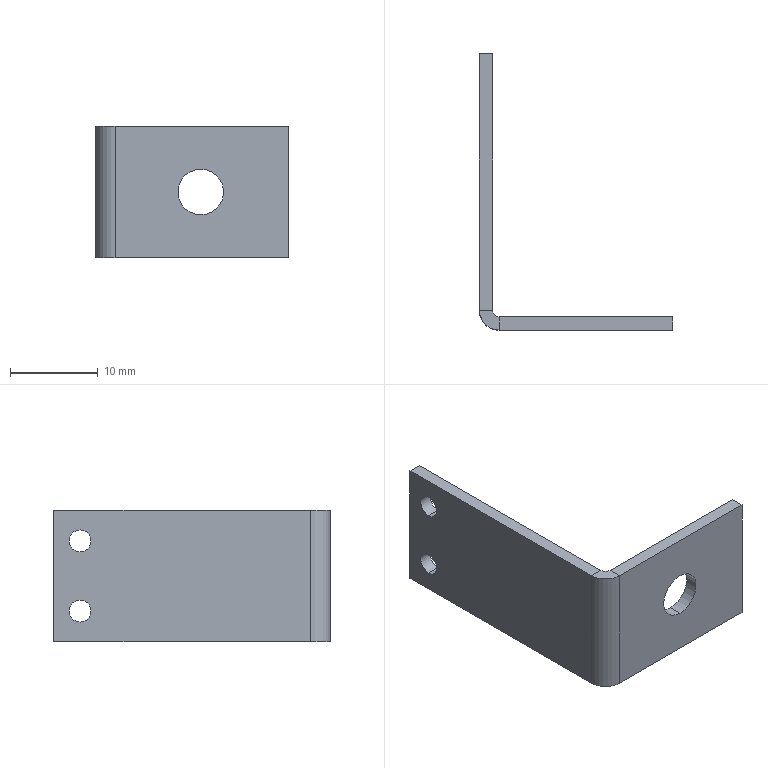Part | SolidWorks | features ICE 2, FlatPattern 1, SMBaseFlange 1, SheetMetal 1 | 1 solid | 20 faces | box 22 x 31.5 x 15 mm | volume 1109 mm3 | plane 12 | cylinder 8 | commonest cylinder face diameters 2.5 x4 5.2 x2 1.473 x1 4.473 x1
STEP:
#1=CARTESIAN_POINT('',(0.,27.,-2.75));
#2=VERTEX_POINT('',#1);
#3=CARTESIAN_POINT('',(0.,27.,-5.25));
#4=VERTEX_POINT('',#3);
#5=CARTESIAN_POINT('',(0.,27.,-4.));
#6=DIRECTION('',(1.,0.,0.));
#7=DIRECTION('',(0.,0.,-1.));
#8=AXIS2_PLACEMENT_3D('',#5,#6,#7);
#9=CIRCLE('',#8,1.25);
#10=EDGE_CURVE('',#2,#4,#9,.T.);
#11=ORIENTED_EDGE('',*,*,#10,.T.);
#12=CARTESIAN_POINT('',(-1.5,27.,-5.25));
#13=VERTEX_POINT('',#12);
#14=CARTESIAN_POINT('',(8.5,27.,-5.25));
#15=DIRECTION('',(-1.,0.,0.));
#16=VECTOR('',#15,1000.);
#17=LINE('',#14,#16);
#18=EDGE_CURVE('',#4,#13,#17,.T.);
#19=ORIENTED_EDGE('',*,*,#18,.T.);
#20=CARTESIAN_POINT('',(-1.5,27.,-2.75));
#21=VERTEX_POINT('',#20);
#22=CARTESIAN_POINT('',(-1.5,27.,-4.));
#23=DIRECTION('',(-1.,0.,0.));
#24=DIRECTION('',(0.,0.,1.));
#25=AXIS2_PLACEMENT_3D('',#22,#23,#24);
#26=CIRCLE('',#25,1.25);
#27=EDGE_CURVE('',#13,#21,#26,.T.);
#28=ORIENTED_EDGE('',*,*,#27,.T.);
#29=CARTESIAN_POINT('',(8.5,27.,-2.75));
#30=DIRECTION('',(-1.,0.,0.));
#31=VECTOR('',#30,1000.);
#32=LINE('',#29,#31);
#33=EDGE_CURVE('',#2,#21,#32,.T.);
#34=ORIENTED_EDGE('',*,*,#33,.F.);
#35=EDGE_LOOP('',(#11,#19,#28,#34));
#36=FACE_OUTER_BOUND('',#35,.T.);
#37=CARTESIAN_POINT('',(8.5,27.,-4.));
#38=DIRECTION('',(-1.,0.,0.));
#39=DIRECTION('',(0.,0.,1.));
#40=AXIS2_PLACEMENT_3D('',#37,#38,#39);
#41=CYLINDRICAL_SURFACE('',#40,1.25);
#42=ADVANCED_FACE('',(#36),#41,.F.);
#43=CARTESIAN_POINT('',(0.,27.,5.25));
#44=VERTEX_POINT('',#43);
#45=CARTESIAN_POINT('',(0.,27.,2.75));
#46=VERTEX_POINT('',#45);
#47=CARTESIAN_POINT('',(0.,27.,4.));
#48=DIRECTION('',(1.,0.,0.));
#49=DIRECTION('',(0.,0.,-1.));
#50=AXIS2_PLACEMENT_3D('',#47,#48,#49);
#51=CIRCLE('',#50,1.25);
#52=EDGE_CURVE('',#44,#46,#51,.T.);
#53=ORIENTED_EDGE('',*,*,#52,.T.);
#54=CARTESIAN_POINT('',(-1.5,27.,2.75));
#55=VERTEX_POINT('',#54);
#56=CARTESIAN_POINT('',(8.5,27.,2.75));
#57=DIRECTION('',(-1.,0.,0.));
#58=VECTOR('',#57,1000.);
#59=LINE('',#56,#58);
#60=EDGE_CURVE('',#46,#55,#59,.T.);
#61=ORIENTED_EDGE('',*,*,#60,.T.);
#62=CARTESIAN_POINT('',(-1.5,27.,5.25));
#63=VERTEX_POINT('',#62);
#64=CARTESIAN_POINT('',(-1.5,27.,4.));
#65=DIRECTION('',(-1.,0.,0.));
#66=DIRECTION('',(0.,0.,-1.));
#67=AXIS2_PLACEMENT_3D('',#64,#65,#66);
#68=CIRCLE('',#67,1.25);
#69=EDGE_CURVE('',#55,#63,#68,.T.);
#70=ORIENTED_EDGE('',*,*,#69,.T.);
#71=CARTESIAN_POINT('',(8.5,27.,5.25));
#72=DIRECTION('',(-1.,0.,0.));
#73=VECTOR('',#72,1000.);
#74=LINE('',#71,#73);
#75=EDGE_CURVE('',#44,#63,#74,.T.);
#76=ORIENTED_EDGE('',*,*,#75,.F.);
#77=EDGE_LOOP('',(#53,#61,#70,#76));
#78=FACE_OUTER_BOUND('',#77,.T.);
#79=CARTESIAN_POINT('',(8.5,27.,4.));
#80=DIRECTION('',(-1.,0.,0.));
#81=DIRECTION('',(0.,0.,1.));
#82=AXIS2_PLACEMENT_3D('',#79,#80,#81);
#83=CYLINDRICAL_SURFACE('',#82,1.25);
#84=ADVANCED_FACE('',(#78),#83,.F.);
#85=CARTESIAN_POINT('',(10.5,0.,-2.6));
#86=VERTEX_POINT('',#85);
#87=CARTESIAN_POINT('',(10.5,0.,2.6));
#88=VERTEX_POINT('',#87);
#89=CARTESIAN_POINT('',(10.5,0.,0.));
#90=DIRECTION('',(0.,1.,0.));
#91=DIRECTION('',(0.,0.,1.));
#92=AXIS2_PLACEMENT_3D('',#89,#90,#91);
#93=CIRCLE('',#92,2.6);
#94=EDGE_CURVE('',#86,#88,#93,.T.);
#95=ORIENTED_EDGE('',*,*,#94,.T.);
#96=CARTESIAN_POINT('',(10.5,-1.5,2.6));
#97=VERTEX_POINT('',#96);
#98=CARTESIAN_POINT('',(10.5,8.5,2.6));
#99=DIRECTION('',(0.,-1.,0.));
#100=VECTOR('',#99,1000.);
#101=LINE('',#98,#100);
#102=EDGE_CURVE('',#88,#97,#101,.T.);
#103=ORIENTED_EDGE('',*,*,#102,.T.);
#104=CARTESIAN_POINT('',(10.5,-1.5,-2.6));
#105=VERTEX_POINT('',#104);
#106=CARTESIAN_POINT('',(10.5,-1.5,0.));
#107=DIRECTION('',(0.,-1.,0.));
#108=DIRECTION('',(0.,0.,-1.));
#109=AXIS2_PLACEMENT_3D('',#106,#107,#108);
#110=CIRCLE('',#109,2.6);
#111=EDGE_CURVE('',#97,#105,#110,.T.);
#112=ORIENTED_EDGE('',*,*,#111,.T.);
#113=CARTESIAN_POINT('',(10.5,8.5,-2.6));
#114=DIRECTION('',(0.,-1.,0.));
#115=VECTOR('',#114,1000.);
#116=LINE('',#113,#115);
#117=EDGE_CURVE('',#86,#105,#116,.T.);
#118=ORIENTED_EDGE('',*,*,#117,.F.);
#119=EDGE_LOOP('',(#95,#103,#112,#118));
#120=FACE_OUTER_BOUND('',#119,.T.);
#121=CARTESIAN_POINT('',(10.5,8.5,0.));
#122=DIRECTION('',(0.,-1.,0.));
#123=DIRECTION('',(0.,0.,-1.));
#124=AXIS2_PLACEMENT_3D('',#121,#122,#123);
#125=CYLINDRICAL_SURFACE('',#124,2.6);
#126=ADVANCED_FACE('',(#120),#125,.F.);
#127=CARTESIAN_POINT('',(0.7366,0.,7.5));
#128=VERTEX_POINT('',#127);
#129=CARTESIAN_POINT('',(0.7366,-1.5,7.5));
#130=VERTEX_POINT('',#129);
#131=CARTESIAN_POINT('',(0.7366,0.,7.5));
#132=DIRECTION('',(0.,-1.,0.));
#133=VECTOR('',#132,1000.);
#134=LINE('',#131,#133);
#135=EDGE_CURVE('',#128,#130,#134,.T.);
#136=ORIENTED_EDGE('',*,*,#135,.F.);
#137=CARTESIAN_POINT('',(0.,0.7366,7.5));
#138=VERTEX_POINT('',#137);
#139=CARTESIAN_POINT('',(0.7366,0.7366,7.5));
#140=DIRECTION('',(0.,0.,1.));
#141=DIRECTION('',(-1.,0.,0.));
#142=AXIS2_PLACEMENT_3D('',#139,#140,#141);
#143=CIRCLE('',#142,0.7366);
#144=EDGE_CURVE('',#138,#128,#143,.T.);
#145=ORIENTED_EDGE('',*,*,#144,.F.);
#146=CARTESIAN_POINT('',(-1.5,0.7366,7.5));
#147=VERTEX_POINT('',#146);
#148=CARTESIAN_POINT('',(-1.5,0.7366,7.5));
#149=DIRECTION('',(1.,0.,0.));
#150=VECTOR('',#149,1000.);
#151=LINE('',#148,#150);
#152=EDGE_CURVE('',#147,#138,#151,.T.);
#153=ORIENTED_EDGE('',*,*,#152,.F.);
#154=CARTESIAN_POINT('',(0.7366,0.7366,7.5));
#155=DIRECTION('',(0.,0.,1.));
#156=DIRECTION('',(1.,0.,0.));
#157=AXIS2_PLACEMENT_3D('',#154,#155,#156);
#158=CIRCLE('',#157,2.237);
#159=EDGE_CURVE('',#147,#130,#158,.T.);
#160=ORIENTED_EDGE('',*,*,#159,.T.);
#161=EDGE_LOOP('',(#136,#145,#153,#160));
#162=FACE_OUTER_BOUND('',#161,.T.);
#163=CARTESIAN_POINT('',(0.7366,0.,7.5));
#164=DIRECTION('',(0.,0.,1.));
#165=DIRECTION('',(1.,0.,0.));
#166=AXIS2_PLACEMENT_3D('',#163,#164,#165);
#167=PLANE('',#166);
#168=ADVANCED_FACE('',(#162),#167,.T.);
#169=CARTESIAN_POINT('',(20.5,0.,7.5));
#170=VERTEX_POINT('',#169);
#171=CARTESIAN_POINT('',(0.,0.,7.5));
#172=DIRECTION('',(1.,0.,0.));
#173=VECTOR('',#172,1000.);
#174=LINE('',#171,#173);
#175=EDGE_CURVE('',#128,#170,#174,.T.);
#176=ORIENTED_EDGE('',*,*,#175,.F.);
#177=ORIENTED_EDGE('',*,*,#135,.T.);
#178=CARTESIAN_POINT('',(20.5,-1.5,7.5));
#179=VERTEX_POINT('',#178);
#180=CARTESIAN_POINT('',(0.,-1.5,7.5));
#181=DIRECTION('',(1.,0.,0.));
#182=VECTOR('',#181,1000.);
#183=LINE('',#180,#182);
#184=EDGE_CURVE('',#130,#179,#183,.T.);
#185=ORIENTED_EDGE('',*,*,#184,.T.);
#186=CARTESIAN_POINT('',(20.5,0.,7.5));
#187=DIRECTION('',(0.,-1.,0.));
#188=VECTOR('',#187,1000.);
#189=LINE('',#186,#188);
#190=EDGE_CURVE('',#170,#179,#189,.T.);
#191=ORIENTED_EDGE('',*,*,#190,.F.);
#192=EDGE_LOOP('',(#176,#177,#185,#191));
#193=FACE_OUTER_BOUND('',#192,.T.);
#194=CARTESIAN_POINT('',(-1.5,0.7366,7.5));
#195=DIRECTION('',(0.,0.,1.));
#196=DIRECTION('',(1.,0.,0.));
#197=AXIS2_PLACEMENT_3D('',#194,#195,#196);
#198=PLANE('',#197);
#199=ADVANCED_FACE('',(#193),#198,.T.);
#200=CARTESIAN_POINT('',(0.,0.7366,-7.5));
#201=VERTEX_POINT('',#200);
#202=CARTESIAN_POINT('',(-1.5,0.7366,-7.5));
#203=VERTEX_POINT('',#202);
#204=CARTESIAN_POINT('',(0.,0.7366,-7.5));
#205=DIRECTION('',(-1.,0.,0.));
#206=VECTOR('',#205,1000.);
#207=LINE('',#204,#206);
#208=EDGE_CURVE('',#201,#203,#207,.T.);
#209=ORIENTED_EDGE('',*,*,#208,.F.);
#210=CARTESIAN_POINT('',(0.7366,0.,-7.5));
#211=VERTEX_POINT('',#210);
#212=CARTESIAN_POINT('',(0.7366,0.7366,-7.5));
#213=DIRECTION('',(0.,0.,1.));
#214=DIRECTION('',(-1.,0.,0.));
#215=AXIS2_PLACEMENT_3D('',#212,#213,#214);
#216=CIRCLE('',#215,0.7366);
#217=EDGE_CURVE('',#201,#211,#216,.T.);
#218=ORIENTED_EDGE('',*,*,#217,.T.);
#219=CARTESIAN_POINT('',(0.7366,-1.5,-7.5));
#220=VERTEX_POINT('',#219);
#221=CARTESIAN_POINT('',(0.7366,-1.5,-7.5));
#222=DIRECTION('',(0.,1.,0.));
#223=VECTOR('',#222,1000.);
#224=LINE('',#221,#223);
#225=EDGE_CURVE('',#220,#211,#224,.T.);
#226=ORIENTED_EDGE('',*,*,#225,.F.);
#227=CARTESIAN_POINT('',(0.7366,0.7366,-7.5));
#228=DIRECTION('',(0.,0.,1.));
#229=DIRECTION('',(1.,0.,0.));
#230=AXIS2_PLACEMENT_3D('',#227,#228,#229);
#231=CIRCLE('',#230,2.237);
#232=EDGE_CURVE('',#203,#220,#231,.T.);
#233=ORIENTED_EDGE('',*,*,#232,.F.);
#234=EDGE_LOOP('',(#209,#218,#226,#233));
#235=FACE_OUTER_BOUND('',#234,.T.);
#236=CARTESIAN_POINT('',(0.,0.7366,-7.5));
#237=DIRECTION('',(0.,0.,-1.));
#238=DIRECTION('',(-1.,0.,0.));
#239=AXIS2_PLACEMENT_3D('',#236,#237,#238);
#240=PLANE('',#239);
#241=ADVANCED_FACE('',(#235),#240,.T.);
#242=CARTESIAN_POINT('',(0.,30.,-7.5));
#243=VERTEX_POINT('',#242);
#244=CARTESIAN_POINT('',(0.,0.,-7.5));
#245=DIRECTION('',(0.,-1.,0.));
#246=VECTOR('',#245,1000.);
#247=LINE('',#244,#246);
#248=EDGE_CURVE('',#243,#201,#247,.T.);
#249=ORIENTED_EDGE('',*,*,#248,.T.);
#250=ORIENTED_EDGE('',*,*,#208,.T.);
#251=CARTESIAN_POINT('',(-1.5,30.,-7.5));
#252=VERTEX_POINT('',#251);
#253=CARTESIAN_POINT('',(-1.5,0.,-7.5));
#254=DIRECTION('',(0.,-1.,0.));
#255=VECTOR('',#254,1000.);
#256=LINE('',#253,#255);
#257=EDGE_CURVE('',#252,#203,#256,.T.);
#258=ORIENTED_EDGE('',*,*,#257,.F.);
#259=CARTESIAN_POINT('',(-1.5,30.,-7.5));
#260=DIRECTION('',(1.,0.,0.));
#261=VECTOR('',#260,1000.);
#262=LINE('',#259,#261);
#263=EDGE_CURVE('',#252,#243,#262,.T.);
#264=ORIENTED_EDGE('',*,*,#263,.T.);
#265=EDGE_LOOP('',(#249,#250,#258,#264));
#266=FACE_OUTER_BOUND('',#265,.T.);
#267=CARTESIAN_POINT('',(0.7366,-1.5,-7.5));
#268=DIRECTION('',(0.,0.,-1.));
#269=DIRECTION('',(-1.,0.,0.));
#270=AXIS2_PLACEMENT_3D('',#267,#268,#269);
#271=PLANE('',#270);
#272=ADVANCED_FACE('',(#266),#271,.T.);
#273=CARTESIAN_POINT('',(10.5,-1.5,0.));
#274=DIRECTION('',(0.,-1.,0.));
#275=DIRECTION('',(0.,0.,-1.));
#276=AXIS2_PLACEMENT_3D('',#273,#274,#275);
#277=CIRCLE('',#276,2.6);
#278=EDGE_CURVE('',#105,#97,#277,.T.);
#279=ORIENTED_EDGE('',*,*,#278,.F.);
#280=ORIENTED_EDGE('',*,*,#111,.F.);
#281=EDGE_LOOP('',(#279,#280));
#282=FACE_BOUND('',#281,.T.);
#283=CARTESIAN_POINT('',(20.5,-1.5,-7.5));
#284=VERTEX_POINT('',#283);
#285=CARTESIAN_POINT('',(0.,-1.5,-7.5));
#286=DIRECTION('',(1.,0.,0.));
#287=VECTOR('',#286,1000.);
#288=LINE('',#285,#287);
#289=EDGE_CURVE('',#220,#284,#288,.T.);
#290=ORIENTED_EDGE('',*,*,#289,.T.);
#291=CARTESIAN_POINT('',(20.5,-1.5,7.5));
#292=DIRECTION('',(0.,0.,-1.));
#293=VECTOR('',#292,1000.);
#294=LINE('',#291,#293);
#295=EDGE_CURVE('',#179,#284,#294,.T.);
#296=ORIENTED_EDGE('',*,*,#295,.F.);
#297=ORIENTED_EDGE('',*,*,#184,.F.);
#298=CARTESIAN_POINT('',(0.7366,-1.5,7.5));
#299=DIRECTION('',(0.,0.,-1.));
#300=VECTOR('',#299,1000.);
#301=LINE('',#298,#300);
#302=EDGE_CURVE('',#130,#220,#301,.T.);
#303=ORIENTED_EDGE('',*,*,#302,.T.);
#304=EDGE_LOOP('',(#290,#296,#297,#303));
#305=FACE_OUTER_BOUND('',#304,.T.);
#306=CARTESIAN_POINT('',(0.,-1.5,7.5));
#307=DIRECTION('',(0.,1.,0.));
#308=DIRECTION('',(0.,0.,1.));
#309=AXIS2_PLACEMENT_3D('',#306,#307,#308);
#310=PLANE('',#309);
#311=ADVANCED_FACE('',(#282,#305),#310,.F.);
#312=CARTESIAN_POINT('',(20.5,0.,-7.5));
#313=VERTEX_POINT('',#312);
#314=CARTESIAN_POINT('',(20.5,0.,-7.5));
#315=DIRECTION('',(0.,-1.,0.));
#316=VECTOR('',#315,1000.);
#317=LINE('',#314,#316);
#318=EDGE_CURVE('',#313,#284,#317,.T.);
#319=ORIENTED_EDGE('',*,*,#318,.F.);
#320=CARTESIAN_POINT('',(20.5,0.,7.5));
#321=DIRECTION('',(0.,0.,-1.));
#322=VECTOR('',#321,1000.);
#323=LINE('',#320,#322);
#324=EDGE_CURVE('',#170,#313,#323,.T.);
#325=ORIENTED_EDGE('',*,*,#324,.F.);
#326=ORIENTED_EDGE('',*,*,#190,.T.);
#327=ORIENTED_EDGE('',*,*,#295,.T.);
#328=EDGE_LOOP('',(#319,#325,#326,#327));
#329=FACE_OUTER_BOUND('',#328,.T.);
#330=CARTESIAN_POINT('',(20.5,0.,7.5));
#331=DIRECTION('',(1.,0.,0.));
#332=DIRECTION('',(0.,0.,-1.));
#333=AXIS2_PLACEMENT_3D('',#330,#331,#332);
#334=PLANE('',#333);
#335=ADVANCED_FACE('',(#329),#334,.T.);
#336=ORIENTED_EDGE('',*,*,#94,.F.);
#337=CARTESIAN_POINT('',(10.5,0.,0.));
#338=DIRECTION('',(0.,1.,0.));
#339=DIRECTION('',(0.,0.,1.));
#340=AXIS2_PLACEMENT_3D('',#337,#338,#339);
#341=CIRCLE('',#340,2.6);
#342=EDGE_CURVE('',#88,#86,#341,.T.);
#343=ORIENTED_EDGE('',*,*,#342,.F.);
#344=EDGE_LOOP('',(#336,#343));
#345=FACE_BOUND('',#344,.T.);
#346=CARTESIAN_POINT('',(0.,0.,-7.5));
#347=DIRECTION('',(1.,0.,0.));
#348=VECTOR('',#347,1000.);
#349=LINE('',#346,#348);
#350=EDGE_CURVE('',#211,#313,#349,.T.);
#351=ORIENTED_EDGE('',*,*,#350,.F.);
#352=CARTESIAN_POINT('',(0.7366,0.,7.5));
#353=DIRECTION('',(0.,0.,-1.));
#354=VECTOR('',#353,1000.);
#355=LINE('',#352,#354);
#356=EDGE_CURVE('',#128,#211,#355,.T.);
#357=ORIENTED_EDGE('',*,*,#356,.F.);
#358=ORIENTED_EDGE('',*,*,#175,.T.);
#359=ORIENTED_EDGE('',*,*,#324,.T.);
#360=EDGE_LOOP('',(#351,#357,#358,#359));
#361=FACE_OUTER_BOUND('',#360,.T.);
#362=CARTESIAN_POINT('',(0.,0.,7.5));
#363=DIRECTION('',(0.,1.,0.));
#364=DIRECTION('',(0.,0.,1.));
#365=AXIS2_PLACEMENT_3D('',#362,#363,#364);
#366=PLANE('',#365);
#367=ADVANCED_FACE('',(#345,#361),#366,.T.);
#368=ORIENTED_EDGE('',*,*,#217,.F.);
#369=CARTESIAN_POINT('',(0.,0.7366,7.5));
#370=DIRECTION('',(0.,0.,-1.));
#371=VECTOR('',#370,1000.);
#372=LINE('',#369,#371);
#373=EDGE_CURVE('',#138,#201,#372,.T.);
#374=ORIENTED_EDGE('',*,*,#373,.F.);
#375=ORIENTED_EDGE('',*,*,#144,.T.);
#376=ORIENTED_EDGE('',*,*,#356,.T.);
#377=EDGE_LOOP('',(#368,#374,#375,#376));
#378=FACE_OUTER_BOUND('',#377,.T.);
#379=CARTESIAN_POINT('',(0.7366,0.7366,7.5));
#380=DIRECTION('',(0.,0.,-1.));
#381=DIRECTION('',(-1.,0.,0.));
#382=AXIS2_PLACEMENT_3D('',#379,#380,#381);
#383=CYLINDRICAL_SURFACE('',#382,0.7366);
#384=ADVANCED_FACE('',(#378),#383,.F.);
#385=ORIENTED_EDGE('',*,*,#10,.F.);
#386=CARTESIAN_POINT('',(0.,27.,-4.));
#387=DIRECTION('',(1.,0.,0.));
#388=DIRECTION('',(0.,0.,-1.));
#389=AXIS2_PLACEMENT_3D('',#386,#387,#388);
#390=CIRCLE('',#389,1.25);
#391=EDGE_CURVE('',#4,#2,#390,.T.);
#392=ORIENTED_EDGE('',*,*,#391,.F.);
#393=EDGE_LOOP('',(#385,#392));
#394=FACE_BOUND('',#393,.T.);
#395=ORIENTED_EDGE('',*,*,#52,.F.);
#396=CARTESIAN_POINT('',(0.,27.,4.));
#397=DIRECTION('',(1.,0.,0.));
#398=DIRECTION('',(0.,0.,-1.));
#399=AXIS2_PLACEMENT_3D('',#396,#397,#398);
#400=CIRCLE('',#399,1.25);
#401=EDGE_CURVE('',#46,#44,#400,.T.);
#402=ORIENTED_EDGE('',*,*,#401,.F.);
#403=EDGE_LOOP('',(#395,#402));
#404=FACE_BOUND('',#403,.T.);
#405=ORIENTED_EDGE('',*,*,#248,.F.);
#406=CARTESIAN_POINT('',(0.,30.,7.5));
#407=VERTEX_POINT('',#406);
#408=CARTESIAN_POINT('',(0.,30.,7.5));
#409=DIRECTION('',(0.,0.,-1.));
#410=VECTOR('',#409,1000.);
#411=LINE('',#408,#410);
#412=EDGE_CURVE('',#407,#243,#411,.T.);
#413=ORIENTED_EDGE('',*,*,#412,.F.);
#414=CARTESIAN_POINT('',(0.,0.,7.5));
#415=DIRECTION('',(0.,-1.,0.));
#416=VECTOR('',#415,1000.);
#417=LINE('',#414,#416);
#418=EDGE_CURVE('',#407,#138,#417,.T.);
#419=ORIENTED_EDGE('',*,*,#418,.T.);
#420=ORIENTED_EDGE('',*,*,#373,.T.);
#421=EDGE_LOOP('',(#405,#413,#419,#420));
#422=FACE_OUTER_BOUND('',#421,.T.);
#423=CARTESIAN_POINT('',(0.,0.,7.5));
#424=DIRECTION('',(1.,0.,0.));
#425=DIRECTION('',(0.,0.,-1.));
#426=AXIS2_PLACEMENT_3D('',#423,#424,#425);
#427=PLANE('',#426);
#428=ADVANCED_FACE('',(#394,#404,#422),#427,.T.);
#429=ORIENTED_EDGE('',*,*,#263,.F.);
#430=CARTESIAN_POINT('',(-1.5,30.,7.5));
#431=VERTEX_POINT('',#430);
#432=CARTESIAN_POINT('',(-1.5,30.,7.5));
#433=DIRECTION('',(0.,0.,-1.));
#434=VECTOR('',#433,1000.);
#435=LINE('',#432,#434);
#436=EDGE_CURVE('',#431,#252,#435,.T.);
#437=ORIENTED_EDGE('',*,*,#436,.F.);
#438=CARTESIAN_POINT('',(-1.5,30.,7.5));
#439=DIRECTION('',(1.,0.,0.));
#440=VECTOR('',#439,1000.);
#441=LINE('',#438,#440);
#442=EDGE_CURVE('',#431,#407,#441,.T.);
#443=ORIENTED_EDGE('',*,*,#442,.T.);
#444=ORIENTED_EDGE('',*,*,#412,.T.);
#445=EDGE_LOOP('',(#429,#437,#443,#444));
#446=FACE_OUTER_BOUND('',#445,.T.);
#447=CARTESIAN_POINT('',(-1.5,30.,7.5));
#448=DIRECTION('',(0.,1.,0.));
#449=DIRECTION('',(0.,0.,1.));
#450=AXIS2_PLACEMENT_3D('',#447,#448,#449);
#451=PLANE('',#450);
#452=ADVANCED_FACE('',(#446),#451,.T.);
#453=CARTESIAN_POINT('',(-1.5,27.,-4.));
#454=DIRECTION('',(-1.,0.,0.));
#455=DIRECTION('',(0.,0.,1.));
#456=AXIS2_PLACEMENT_3D('',#453,#454,#455);
#457=CIRCLE('',#456,1.25);
#458=EDGE_CURVE('',#21,#13,#457,.T.);
#459=ORIENTED_EDGE('',*,*,#458,.F.);
#460=ORIENTED_EDGE('',*,*,#27,.F.);
#461=EDGE_LOOP('',(#459,#460));
#462=FACE_BOUND('',#461,.T.);
#463=CARTESIAN_POINT('',(-1.5,27.,4.));
#464=DIRECTION('',(-1.,0.,0.));
#465=DIRECTION('',(0.,0.,-1.));
#466=AXIS2_PLACEMENT_3D('',#463,#464,#465);
#467=CIRCLE('',#466,1.25);
#468=EDGE_CURVE('',#63,#55,#467,.T.);
#469=ORIENTED_EDGE('',*,*,#468,.F.);
#470=ORIENTED_EDGE('',*,*,#69,.F.);
#471=EDGE_LOOP('',(#469,#470));
#472=FACE_BOUND('',#471,.T.);
#473=ORIENTED_EDGE('',*,*,#257,.T.);
#474=CARTESIAN_POINT('',(-1.5,0.7366,7.5));
#475=DIRECTION('',(0.,0.,-1.));
#476=VECTOR('',#475,1000.);
#477=LINE('',#474,#476);
#478=EDGE_CURVE('',#147,#203,#477,.T.);
#479=ORIENTED_EDGE('',*,*,#478,.F.);
#480=CARTESIAN_POINT('',(-1.5,0.,7.5));
#481=DIRECTION('',(0.,-1.,0.));
#482=VECTOR('',#481,1000.);
#483=LINE('',#480,#482);
#484=EDGE_CURVE('',#431,#147,#483,.T.);
#485=ORIENTED_EDGE('',*,*,#484,.F.);
#486=ORIENTED_EDGE('',*,*,#436,.T.);
#487=EDGE_LOOP('',(#473,#479,#485,#486));
#488=FACE_OUTER_BOUND('',#487,.T.);
#489=CARTESIAN_POINT('',(-1.5,0.,7.5));
#490=DIRECTION('',(1.,0.,0.));
#491=DIRECTION('',(0.,0.,-1.));
#492=AXIS2_PLACEMENT_3D('',#489,#490,#491);
#493=PLANE('',#492);
#494=ADVANCED_FACE('',(#462,#472,#488),#493,.F.);
#495=ORIENTED_EDGE('',*,*,#232,.T.);
#496=ORIENTED_EDGE('',*,*,#302,.F.);
#497=ORIENTED_EDGE('',*,*,#159,.F.);
#498=ORIENTED_EDGE('',*,*,#478,.T.);
#499=EDGE_LOOP('',(#495,#496,#497,#498));
#500=FACE_OUTER_BOUND('',#499,.T.);
#501=CARTESIAN_POINT('',(0.7366,0.7366,7.5));
#502=DIRECTION('',(0.,0.,-1.));
#503=DIRECTION('',(-1.,0.,0.));
#504=AXIS2_PLACEMENT_3D('',#501,#502,#503);
#505=CYLINDRICAL_SURFACE('',#504,2.237);
#506=ADVANCED_FACE('',(#500),#505,.T.);
#507=ORIENTED_EDGE('',*,*,#484,.T.);
#508=ORIENTED_EDGE('',*,*,#152,.T.);
#509=ORIENTED_EDGE('',*,*,#418,.F.);
#510=ORIENTED_EDGE('',*,*,#442,.F.);
#511=EDGE_LOOP('',(#507,#508,#509,#510));
#512=FACE_OUTER_BOUND('',#511,.T.);
#513=CARTESIAN_POINT('',(0.7366,0.7366,7.5));
#514=DIRECTION('',(0.,0.,-1.));
#515=DIRECTION('',(-1.,0.,0.));
#516=AXIS2_PLACEMENT_3D('',#513,#514,#515);
#517=PLANE('',#516);
#518=ADVANCED_FACE('',(#512),#517,.F.);
#519=ORIENTED_EDGE('',*,*,#289,.F.);
#520=ORIENTED_EDGE('',*,*,#225,.T.);
#521=ORIENTED_EDGE('',*,*,#350,.T.);
#522=ORIENTED_EDGE('',*,*,#318,.T.);
#523=EDGE_LOOP('',(#519,#520,#521,#522));
#524=FACE_OUTER_BOUND('',#523,.T.);
#525=CARTESIAN_POINT('',(0.7366,0.7366,-7.5));
#526=DIRECTION('',(0.,0.,-1.));
#527=DIRECTION('',(-1.,0.,0.));
#528=AXIS2_PLACEMENT_3D('',#525,#526,#527);
#529=PLANE('',#528);
#530=ADVANCED_FACE('',(#524),#529,.T.);
#531=ORIENTED_EDGE('',*,*,#102,.F.);
#532=ORIENTED_EDGE('',*,*,#342,.T.);
#533=ORIENTED_EDGE('',*,*,#117,.T.);
#534=ORIENTED_EDGE('',*,*,#278,.T.);
#535=EDGE_LOOP('',(#531,#532,#533,#534));
#536=FACE_OUTER_BOUND('',#535,.T.);
#537=CARTESIAN_POINT('',(10.5,8.5,0.));
#538=DIRECTION('',(0.,-1.,0.));
#539=DIRECTION('',(0.,0.,-1.));
#540=AXIS2_PLACEMENT_3D('',#537,#538,#539);
#541=CYLINDRICAL_SURFACE('',#540,2.6);
#542=ADVANCED_FACE('',(#536),#541,.F.);
#543=ORIENTED_EDGE('',*,*,#60,.F.);
#544=ORIENTED_EDGE('',*,*,#401,.T.);
#545=ORIENTED_EDGE('',*,*,#75,.T.);
#546=ORIENTED_EDGE('',*,*,#468,.T.);
#547=EDGE_LOOP('',(#543,#544,#545,#546));
#548=FACE_OUTER_BOUND('',#547,.T.);
#549=CARTESIAN_POINT('',(8.5,27.,4.));
#550=DIRECTION('',(-1.,0.,0.));
#551=DIRECTION('',(0.,0.,1.));
#552=AXIS2_PLACEMENT_3D('',#549,#550,#551);
#553=CYLINDRICAL_SURFACE('',#552,1.25);
#554=ADVANCED_FACE('',(#548),#553,.F.);
#555=ORIENTED_EDGE('',*,*,#18,.F.);
#556=ORIENTED_EDGE('',*,*,#391,.T.);
#557=ORIENTED_EDGE('',*,*,#33,.T.);
#558=ORIENTED_EDGE('',*,*,#458,.T.);
#559=EDGE_LOOP('',(#555,#556,#557,#558));
#560=FACE_OUTER_BOUND('',#559,.T.);
#561=CARTESIAN_POINT('',(8.5,27.,-4.));
#562=DIRECTION('',(-1.,0.,0.));
#563=DIRECTION('',(0.,0.,1.));
#564=AXIS2_PLACEMENT_3D('',#561,#562,#563);
#565=CYLINDRICAL_SURFACE('',#564,1.25);
#566=ADVANCED_FACE('',(#560),#565,.F.);
#567=CLOSED_SHELL('',(#42,#84,#126,#168,#199,#241,#272,#311,#335,#367,#384,#428,#452,#494,#506,#518,#530,#542,#554,#566));
#568=MANIFOLD_SOLID_BREP('',#567);
#569=CARTESIAN_POINT('',(0.,0.,0.));
#570=DIRECTION('',(0.,0.,1.));
#571=DIRECTION('',(1.,0.,0.));
#572=AXIS2_PLACEMENT_3D('',#569,#570,#571);
#573=(LENGTH_UNIT()NAMED_UNIT(*)SI_UNIT(.MILLI.,.METRE.));
#574=UNCERTAINTY_MEASURE_WITH_UNIT(LENGTH_MEASURE(0.00001),#573,'','');
#575=(NAMED_UNIT(*)PLANE_ANGLE_UNIT()SI_UNIT($,.RADIAN.));
#576=(NAMED_UNIT(*)SI_UNIT($,.STERADIAN.)SOLID_ANGLE_UNIT());
#577=(GEOMETRIC_REPRESENTATION_CONTEXT(3)GLOBAL_UNCERTAINTY_ASSIGNED_CONTEXT((#574))GLOBAL_UNIT_ASSIGNED_CONTEXT((#573,#575,#576))REPRESENTATION_CONTEXT('',''));
#578=ADVANCED_BREP_SHAPE_REPRESENTATION('',(#568,#572),#577);